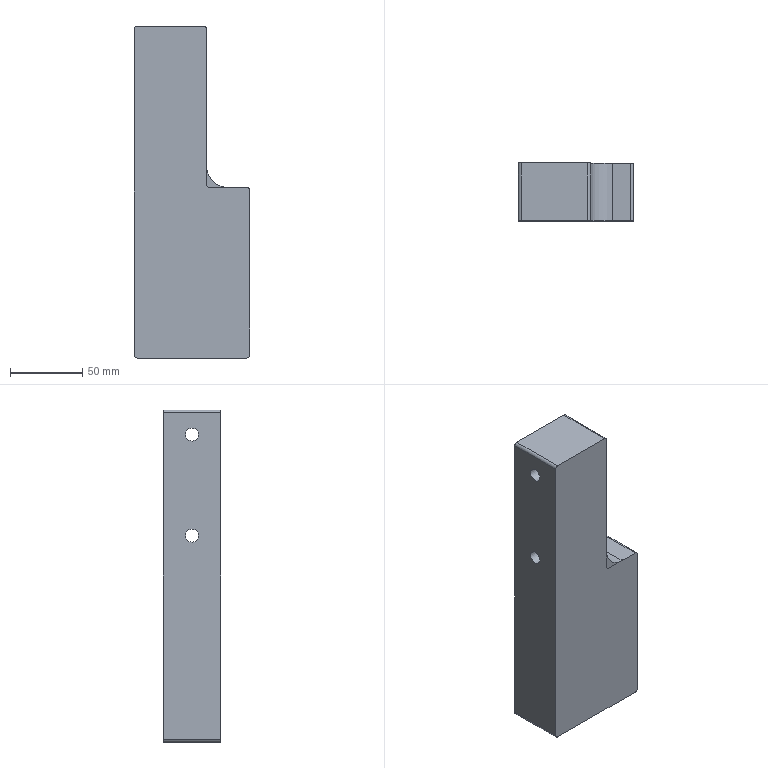NC program | NX | posted with a generic post | part box 80 x 40 x 230 mm
Whole program:
N10 G17 G21 G94 G90
(DRILLING_COPY , TOOL : D8点钻)
N12 T03 M6
N14 G53
N16 G17 G0 G90 X16. Y-10.9 B0. C0. S3500 M3
N18 G43 Z30. H3
N20 G94 G81 G98 Z-4.2 B-180. C-90. F300. R3.
N22 X106.
N24 X143. Y-20. Z-34.1 R-26.9
N26 X213.
N28 G80
N30 G0 X213. Y-20. Z30.
N32 M5
(PECK_DRILLING , TOOL : Z6.8)
N34 T10 M6
N36 G53
N38 G17 G0 G90 X16. Y-10.9 B0. C0. S1200 M3
N40 G43 Z50. H10
N42 G94 G83 G99 Z-33. B-180. C-90. F80. Q2. R3.
N44 X106.
N46 G80
N48 G0 X106. Y-10.9 Z50.
N50 M5
(PECK_DRILLING_COPY_1 , TOOL : Z9.)
N52 T24 M6
N54 G53
N56 G17 G0 G90 X143. Y-20. B0. C0. S1000 M3
N58 G43 Z50. H24
N60 G94 G83 G99 Z-85.9 B-180. C-90. F80. Q2. R-26.9
N62 X213.
N64 G80
N66 G0 X213. Y-20. Z50.
N68 M5
(HOLE_MILLING , TOOL : D6.)
N70 T05 M6
N72 G53
N74 G17 G0 G90 X143. Y-20. B0. C0. S2700 M3
N76 G43 Z50. H5
N78 Z-29.4 B-180. C-90.
N80 G94 G3 X140.765 Y-22.235 R2.235 F800.
N82 X143. Y-24.47 R2.235
N84 X143. Y-24.47 Z-29.65 I0. J4.47
N86 X143. Y-24.47 Z-29.9 I0. J4.47
N88 X143. Y-24.47 Z-30.15 I0. J4.47
N90 X143. Y-24.47 Z-30.4 I0. J4.47
N92 X143. Y-24.47 Z-30.65 I0. J4.47
N94 X143. Y-24.47 Z-30.9 I0. J4.47
N96 X143. Y-24.47 Z-31.15 I0. J4.47
N98 X143. Y-24.47 Z-31.4 I0. J4.47
N100 X143. Y-24.47 Z-31.65 I0. J4.47
N102 X143. Y-24.47 Z-31.9 I0. J4.47
N104 X143. Y-24.47 Z-32.15 I0. J4.47
N106 X143. Y-24.47 Z-32.4 I0. J4.47
N108 X143. Y-24.47 Z-32.65 I0. J4.47
N110 X143. Y-24.47 Z-32.9 I0. J4.47
N112 X143. Y-24.47 Z-33.15 I0. J4.47
N114 X143. Y-24.47 Z-33.4 I0. J4.47
N116 X143. Y-24.47 Z-33.65 I0. J4.47
N118 X143. Y-24.47 Z-33.9 I0. J4.47
N120 X143. Y-24.47 Z-34.15 I0. J4.47
N122 X143. Y-24.47 Z-34.4 I0. J4.47
N124 X143. Y-24.47 Z-34.65 I0. J4.47
N126 X143. Y-24.47 Z-34.9 I0. J4.47
N128 X143. Y-24.47 Z-35.15 I0. J4.47
N130 X143. Y-24.47 Z-35.4 I0. J4.47
N132 X143. Y-24.47 Z-35.65 I0. J4.47
N134 X143. Y-24.47 Z-35.9 I0. J4.47
N136 X143. Y-24.47 Z-36.15 I0. J4.47
N138 X143. Y-24.47 Z-36.4 I0. J4.47
N140 X143. Y-24.47 Z-36.65 I0. J4.47
N142 X143. Y-24.47 Z-36.9 I0. J4.47
N144 X143. Y-24.47 Z-37.15 I0. J4.47
N146 X143. Y-24.47 Z-37.4 I0. J4.47
N148 X143. Y-24.47 Z-37.65 I0. J4.47
N150 X143. Y-24.47 Z-37.9 I0. J4.47
N152 X143. Y-24.47 Z-38.15 I0. J4.47
N154 X143. Y-24.47 Z-38.4 I0. J4.47
N156 X143. Y-24.47 Z-38.65 I0. J4.47
N158 X143. Y-24.47 Z-38.9 I0. J4.47
N160 X143. Y-24.47 Z-39.15 I0. J4.47
N162 X143. Y-24.47 Z-39.4 I0. J4.47
N164 X143. Y-24.47 Z-39.65 I0. J4.47
N166 X143. Y-24.47 Z-39.9 I0. J4.47
N168 X143. Y-24.47 Z-40.15 I0. J4.47
N170 X143. Y-24.47 Z-40.4 I0. J4.47
N172 X143. Y-24.47 Z-40.65 I0. J4.47
N174 X143. Y-24.47 Z-40.9 I0. J4.47
N176 X143. Y-24.47 Z-41.15 I0. J4.47
N178 X143. Y-24.47 Z-41.4 I0. J4.47
N180 X143. Y-24.47 Z-41.65 I0. J4.47
N182 X143. Y-24.47 Z-41.9 I0. J4.47
N184 X143. Y-24.47 Z-42.15 I0. J4.47
N186 X143. Y-24.47 Z-42.4 I0. J4.47
N188 X143. Y-24.47 Z-42.65 I0. J4.47
N190 X143. Y-24.47 Z-42.9 I0. J4.47
N192 X143. Y-24.47 Z-43.15 I0. J4.47
N194 X143. Y-24.47 Z-43.4 I0. J4.47
N196 X143. Y-24.47 Z-43.65 I0. J4.47
N198 X143. Y-24.47 Z-43.9 I0. J4.47
N200 X143. Y-24.47 Z-44.15 I0. J4.47
N202 X143. Y-24.47 Z-44.4 I0. J4.47
N204 X143. Y-24.47 Z-44.65 I0. J4.47
N206 X143. Y-24.47 Z-44.9 I0. J4.47
N208 X147.251 Y-21.381 Z-44.95 R4.47
N210 X144.381 Y-15.749 R4.47
N212 X147.251 Y-21.381 R-4.47
N214 X145.816 Y-18.565 R2.235
N216 X143. Y-20. R2.235
N218 G0 Z50.
N220 X213.
N222 Z-29.4
N224 G3 X210.765 Y-22.235 R2.235
N226 X213. Y-24.47 R2.235
N228 X213. Y-24.47 Z-29.65 I0. J4.47
N230 X213. Y-24.47 Z-29.9 I0. J4.47
N232 X213. Y-24.47 Z-30.15 I0. J4.47
N234 X213. Y-24.47 Z-30.4 I0. J4.47
N236 X213. Y-24.47 Z-30.65 I0. J4.47
N238 X213. Y-24.47 Z-30.9 I0. J4.47
N240 X213. Y-24.47 Z-31.15 I0. J4.47
N242 X213. Y-24.47 Z-31.4 I0. J4.47
N244 X213. Y-24.47 Z-31.65 I0. J4.47
N246 X213. Y-24.47 Z-31.9 I0. J4.47
N248 X213. Y-24.47 Z-32.15 I0. J4.47
N250 X213. Y-24.47 Z-32.4 I0. J4.47
N252 X213. Y-24.47 Z-32.65 I0. J4.47
N254 X213. Y-24.47 Z-32.9 I0. J4.47
N256 X213. Y-24.47 Z-33.15 I0. J4.47
N258 X213. Y-24.47 Z-33.4 I0. J4.47
N260 X213. Y-24.47 Z-33.65 I0. J4.47
N262 X213. Y-24.47 Z-33.9 I0. J4.47
N264 X213. Y-24.47 Z-34.15 I0. J4.47
N266 X213. Y-24.47 Z-34.4 I0. J4.47
N268 X213. Y-24.47 Z-34.65 I0. J4.47
N270 X213. Y-24.47 Z-34.9 I0. J4.47
N272 X213. Y-24.47 Z-35.15 I0. J4.47
N274 X213. Y-24.47 Z-35.4 I0. J4.47
N276 X213. Y-24.47 Z-35.65 I0. J4.47
N278 X213. Y-24.47 Z-35.9 I0. J4.47
N280 X213. Y-24.47 Z-36.15 I0. J4.47
N282 X213. Y-24.47 Z-36.4 I0. J4.47
N284 X213. Y-24.47 Z-36.65 I0. J4.47
N286 X213. Y-24.47 Z-36.9 I0. J4.47
N288 X213. Y-24.47 Z-37.15 I0. J4.47
N290 X213. Y-24.47 Z-37.4 I0. J4.47
N292 X213. Y-24.47 Z-37.65 I0. J4.47
N294 X213. Y-24.47 Z-37.9 I0. J4.47
N296 X213. Y-24.47 Z-38.15 I0. J4.47
N298 X213. Y-24.47 Z-38.4 I0. J4.47
N300 X213. Y-24.47 Z-38.65 I0. J4.47
N302 X213. Y-24.47 Z-38.9 I0. J4.47
N304 X213. Y-24.47 Z-39.15 I0. J4.47
N306 X213. Y-24.47 Z-39.4 I0. J4.47
N308 X213. Y-24.47 Z-39.65 I0. J4.47
N310 X213. Y-24.47 Z-39.9 I0. J4.47
N312 X213. Y-24.47 Z-40.15 I0. J4.47
N314 X213. Y-24.47 Z-40.4 I0. J4.47
N316 X213. Y-24.47 Z-40.65 I0. J4.47
N318 X213. Y-24.47 Z-40.9 I0. J4.47
N320 X213. Y-24.47 Z-41.15 I0. J4.47
N322 X213. Y-24.47 Z-41.4 I0. J4.47
N324 X213. Y-24.47 Z-41.65 I0. J4.47
N326 X213. Y-24.47 Z-41.9 I0. J4.47
N328 X213. Y-24.47 Z-42.15 I0. J4.47
N330 X213. Y-24.47 Z-42.4 I0. J4.47
N332 X213. Y-24.47 Z-42.65 I0. J4.47
N334 X213. Y-24.47 Z-42.9 I0. J4.47
N336 X213. Y-24.47 Z-43.15 I0. J4.47
N338 X213. Y-24.47 Z-43.4 I0. J4.47
N340 X213. Y-24.47 Z-43.65 I0. J4.47
N342 X213. Y-24.47 Z-43.9 I0. J4.47
N344 X213. Y-24.47 Z-44.15 I0. J4.47
N346 X213. Y-24.47 Z-44.4 I0. J4.47
N348 X213. Y-24.47 Z-44.65 I0. J4.47
N350 X213. Y-24.47 Z-44.9 I0. J4.47
N352 X217.251 Y-21.381 Z-44.95 R4.47
N354 X214.381 Y-15.749 R4.47
N356 X217.251 Y-21.381 R-4.47
N358 X215.816 Y-18.565 R2.235
N360 X213. Y-20. R2.235
N362 G0 Z50.
(HOLE_MILLING_COPY , TOOL : D6.)
N364 X143. S3000
N366 Z-45.
N368 G3 X140.75 Y-22.25 R2.25 F60.
N370 X143. Y-24.5 R2.25
N372 X147.5 Y-20. R4.5
N374 X143. Y-24.5 R-4.5
N376 X145.25 Y-22.25 R2.25
N378 X143. Y-20. R2.25
N380 G0 Z50.
N382 X213.
N384 Z-45.
N386 G3 X210.75 Y-22.25 R2.25
N388 X213. Y-24.5 R2.25
N390 X217.5 Y-20. R4.5
N392 X213. Y-24.5 R-4.5
N394 X215.25 Y-22.25 R2.25
N396 X213. Y-20. R2.25
N398 G0 Z50.
N400 M5
(ZLEVEL_PROFILE_STEEP , TOOL : D16CU)
N402 T01 M6
N404 G53
N406 G17 G0 G90 X126.2 Y10.296 B0. C0. S2600 M3
N408 G43 Z50. H1
N410 Z-15.199 B-180. C-90.
N412 G94 G1 Y0. F2200.
N414 Y-40.
N416 Y-50.296
N418 G0 Z-15.397
N420 G1 Y-40.
N422 Y0.
N424 Y10.296
N426 G0 Z-15.596
N428 G1 Y0.
N430 Y-40.
N432 Y-50.296
N434 G0 Z-15.795
N436 G1 Y-40.
N438 Y0.
N440 Y10.296
N442 G0 Z-15.993
N444 G1 Y0.
N446 Y-40.
N448 Y-50.296
N450 G0 Z-16.192
N452 G1 Y-40.
N454 Y0.
N456 Y10.296
N458 G0 Z-16.391
N460 G1 Y0.
N462 Y-40.
N464 Y-50.296
N466 G0 Z-16.589
N468 G1 Y-40.
N470 Y0.
N472 Y10.296
N474 G0 Z-16.788
N476 G1 Y0.
N478 Y-40.
N480 Y-50.296
N482 G0 Z-16.987
N484 G1 Y-40.
N486 Y0.
N488 Y10.296
N490 G0 Z-17.185
N492 G1 Y0.
N494 Y-40.
N496 Y-50.296
N498 G0 Z-17.384
N500 G1 Y-40.
N502 Y0.
N504 Y10.296
N506 G0 Z-17.583
N508 G1 Y0.
N510 Y-40.
N512 Y-50.296
N514 G0 Z-17.781
N516 G1 Y-40.
N518 Y0.
N520 Y10.296
N522 G0 Z-17.98
N524 G1 Y0.
N526 Y-40.
N528 Y-50.296
N530 G0 Z-18.179
N532 G1 Y-40.
N534 Y0.
N536 Y10.296
N538 G0 Z-18.377
N540 G1 Y0.
N542 Y-40.
N544 Y-50.296
N546 G0 Z-18.576
N548 G1 Y-40.
N550 Y0.
N552 Y10.296
N554 G0 Z-18.775
N556 G1 Y0.
N558 Y-40.
N560 Y-50.296
N562 G0 Z-18.973
N564 G1 Y-40.
N566 Y0.
N568 Y10.296
N570 G0 Z-19.172
N572 G1 Y0.
N574 Y-40.
N576 Y-50.296
N578 G0 Z-19.371
N580 G1 Y-40.
N582 Y0.
N584 Y10.296
N586 G0 Z-19.569
N588 G1 Y0.
N590 Y-40.
N592 Y-50.296
N594 G0 Z-19.768
N596 G1 Y-40.
N598 Y0.
N600 Y10.296
N602 G0 Z-19.967
N604 G1 Y0.
N606 Y-40.
N608 Y-50.296
N610 G0 Z-20.165
N612 G1 Y-40.
N614 Y0.
N616 Y10.296
N618 G0 Z-20.364
N620 G1 Y0.
N622 Y-40.
N624 Y-50.296
N626 G0 Z-20.563
N628 G1 Y-40.
N630 Y0.
N632 Y10.296
N634 G0 Z-20.761
N636 G1 Y0.
N638 Y-40.
N640 Y-50.296
N642 G0 Z-20.96
N644 G1 Y-40.
N646 Y0.
N648 Y10.296
N650 G0 Z-21.159
N652 G1 Y0.
N654 Y-40.
N656 Y-50.296
N658 G0 Z-21.357
N660 G1 Y-40.
N662 Y0.
N664 Y10.296
N666 G0 Z-21.556
N668 G1 Y0.
N670 Y-40.
N672 Y-50.296
N674 G0 Z-21.755
N676 G1 Y-40.
N678 Y0.
N680 Y10.296
N682 G0 Z-21.953
N684 G1 Y0.
N686 Y-40.
N688 Y-50.296
N690 G0 Z-22.152
N692 G1 Y-40.
N694 Y0.
N696 Y10.296
N698 G0 Z-22.351
N700 G1 Y0.
N702 Y-40.
N704 Y-50.296
N706 G0 Z-22.549
N708 G1 Y-40.
N710 Y0.
N712 Y10.296
N714 G0 Z-22.748
N716 G1 Y0.
N718 Y-40.
N720 Y-50.296
N722 G0 Z-22.947
N724 G1 Y-40.
N726 Y0.
N728 Y10.296
N730 G0 Z-23.145
N732 G1 Y0.
N734 Y-40.
N736 Y-50.296
N738 G0 Z-23.344
N740 G1 Y-40.
N742 Y0.
N744 Y10.296
N746 G0 Z-23.543
N748 G1 Y0.
N750 Y-40.
N752 Y-50.296
N754 G0 Z-23.741
N756 G1 Y-40.
N758 Y0.
N760 Y10.296
N762 G0 Z-23.94
N764 G1 Y0.
N766 Y-40.
N768 Y-50.296
N770 G0 Z-24.139
N772 G1 Y-40.
N774 Y0.
N776 Y10.296
N778 G0 Z-24.337
N780 G1 Y0.
N782 Y-40.
N784 Y-50.296
N786 G0 Z-24.536
N788 G1 Y-40.
N790 Y0.
N792 Y10.296
N794 G0 Z-24.735
N796 G1 Y0.
N798 Y-40.
N800 Y-50.296
N802 G0 Z-24.933
N804 G1 Y-40.
N806 Y0.
N808 Y10.296
N810 G0 Z-25.132
N812 G1 Y0.
N814 Y-40.
N816 Y-50.296
N818 G0 Z-25.331
N820 G1 Y-40.
N822 Y0.
N824 Y10.296
N826 G0 Z-25.529
N828 G1 Y0.
N830 Y-40.
N832 Y-50.296
N834 G0 Z-25.728
N836 G1 Y-40.
N838 Y0.
N840 Y10.296
N842 G0 Z-25.927
N844 G1 Y0.
N846 Y-40.
N848 Y-50.296
N850 G0 Z-26.125
N852 G1 Y-40.
N854 Y0.
N856 Y10.296
N858 G0 Z-26.324
N860 G1 Y0.
N862 Y-40.
N864 Y-50.296
N866 G0 Z-26.523
N868 G1 Y-40.
N870 Y0.
N872 Y10.296
N874 G0 Z-26.721
N876 G1 Y0.
N878 Y-40.
N880 Y-50.296
N882 G0 Z-26.92
N884 G1 Y-40.
N886 Y0.
N888 Y10.296
N890 G0 Z-27.119
N892 G1 Y0.
N894 Y-40.
N896 Y-50.296
N898 G0 Z-27.317
N900 G1 Y-40.
N902 Y0.
N904 Y10.296
N906 G0 Z-27.516
N908 G1 Y0.
N910 Y-40.
N912 Y-50.296
N914 G0 Z-27.715
N916 G1 Y-40.
N918 Y0.
N920 Y10.296
N922 G0 Y10.297 Z-27.913
N924 G1 Y-0.069
N926 Y-39.925
N928 Y-50.297
N930 G0 X126.218 Y-50.306 Z-28.112
N932 G1 Y-39.981
N934 X126.212 Y-39.963
N936 Y-0.011
N938 Y10.315
N940 G0 X126.245 Y10.317 Z-28.311
N942 G1 Y0.
N944 Y-40.
N946 Y-50.314
N948 G0 X126.3 Y-50.306 Z-28.509
N950 G1 Y-40.
N952 Y0.
N954 Y10.301
N956 G0 X126.38 Y10.331 Z-28.708
N958 G1 Y-0.072
N960 Y-39.922
N962 Y-50.33
N964 G0 X126.489 Y-50.311 Z-28.907
N966 G1 Y-40.
N968 Y0.002
N970 Y10.326
N972 G0 X126.631 Y10.321 Z-29.105
N974 G1 Y0.
N976 Y-40.
N978 Y-50.316
N980 G0 X126.82 Y-50.322 Z-29.304
N982 G1 Y-40.
N984 Y0.
N986 Y10.319
N988 G0 X127.079 Y10.315 Z-29.503
N990 G1 Y0.
N992 Y-40.
N994 Y-50.319
N996 G0 X127.496 Y-50.32 Z-29.701
N998 G1 Y-40.
N1000 Y0.
N1002 Y10.309
N1004 G0 Z50.
N1006 M5
(PLANAR_MILL , TOOL : D10R2.)
N1008 T23 M6
N1010 G53
N1012 G17 G0 G90 X123.12 Y10. B0. C0. S2400 M3
N1014 G43 Z50. H23
N1016 Z-11.9 B-180. C-90.
N1018 G94 G1 Z-14.9 F400.
N1020 Y0.
N1022 Y-40.
N1024 Y-50.
N1026 Z-11.9
N1028 G0 Z50.
N1030 X123.1 Y10.
N1032 Z-11.9
N1034 G1 Z-14.9
N1036 Y0.
N1038 Y-40.
N1040 Y-50.
N1042 Z-11.9
N1044 G0 Z50.
(PLANAR_MILL_COPY_2 , TOOL : D10R2.)
N1046 X123.125 Y10.
N1048 Z-26.9
N1050 G1 Z-29.9
N1052 Y0.
N1054 Y-40.
N1056 Y-50.
N1058 Z-26.9
N1060 G0 Z50.
N1062 X123.105 Y10.
N1064 Z-26.9
N1066 G1 Z-29.9
N1068 Y0.
N1070 Y-40.
N1072 Y-50.
N1074 Z-26.9
N1076 G0 Z50.
(PLANAR_MILL_COPY_1 , TOOL : D10R2.)
N1078 X228.105 Y8.
N1080 Z-29.7
N1082 G1 Z-29.9
N1084 Y0.
N1086 Y-40.
N1088 Y-48.
N1090 Z-29.7
N1092 G0 X223.105 Y8.
N1094 G1 Z-29.9
N1096 Y0.
N1098 Y-40.
N1100 Y-48.
N1102 Z-29.7
N1104 G0 X218.105 Y8.
N1106 G1 Z-29.9
N1108 Y0.
N1110 Y-40.
N1112 Y-48.
N1114 Z-29.7
N1116 G0 X213.105 Y8.
N1118 G1 Z-29.9
N1120 Y0.
N1122 Y-40.
N1124 Y-48.
N1126 Z-29.7
N1128 G0 X208.105 Y8.
N1130 G1 Z-29.9
N1132 Y0.
N1134 Y-40.
N1136 Y-48.
N1138 Z-29.7
N1140 G0 X203.105 Y8.
N1142 G1 Z-29.9
N1144 Y0.
N1146 Y-40.
N1148 Y-48.
N1150 Z-29.7
N1152 G0 X198.105 Y8.
N1154 G1 Z-29.9
N1156 Y0.
N1158 Y-40.
N1160 Y-48.
N1162 Z-29.7
N1164 G0 X193.105 Y8.
N1166 G1 Z-29.9
N1168 Y0.
N1170 Y-40.
N1172 Y-48.
N1174 Z-29.7
N1176 G0 X188.105 Y8.
N1178 G1 Z-29.9
N1180 Y0.
N1182 Y-40.
N1184 Y-48.
N1186 Z-29.7
N1188 G0 X183.105 Y8.
N1190 G1 Z-29.9
N1192 Y0.
N1194 Y-40.
N1196 Y-48.
N1198 Z-29.7
N1200 G0 X178.105 Y8.
N1202 G1 Z-29.9
N1204 Y0.
N1206 Y-40.
N1208 Y-48.
N1210 Z-29.7
N1212 G0 X173.105 Y8.
N1214 G1 Z-29.9
N1216 Y0.
N1218 Y-40.
N1220 Y-48.
N1222 Z-29.7
N1224 G0 X168.105 Y8.
N1226 G1 Z-29.9
N1228 Y0.
N1230 Y-40.
N1232 Y-48.
N1234 Z-29.7
N1236 G0 X163.105 Y8.
N1238 G1 Z-29.9
N1240 Y0.
N1242 Y-40.
N1244 Y-48.
N1246 Z-29.7
N1248 G0 X158.105 Y8.
N1250 G1 Z-29.9
N1252 Y0.
N1254 Y-40.
N1256 Y-48.
N1258 Z-29.7
N1260 G0 X153.105 Y8.
N1262 G1 Z-29.9
N1264 Y0.
N1266 Y-40.
N1268 Y-48.
N1270 Z-29.7
N1272 G0 X148.105 Y8.
N1274 G1 Z-29.9
N1276 Y0.
N1278 Y-40.
N1280 Y-48.
N1282 Z-29.7
N1284 G0 X143.105 Y8.
N1286 G1 Z-29.9
N1288 Y0.
N1290 Y-40.
N1292 Y-48.
N1294 Z-29.7
N1296 G0 X138.105 Y8.
N1298 G1 Z-29.9
N1300 Y0.
N1302 Y-40.
N1304 Y-48.
N1306 Z-29.7
N1308 G0 X133.105 Y8.
N1310 G1 Z-29.9
N1312 Y0.
N1314 Y-40.
N1316 Y-48.
N1318 Z-29.7
N1320 G0 X128.105 Y8.
N1322 G1 Z-29.9
N1324 Y0.
N1326 Y-40.
N1328 Y-48.
N1330 Z-29.7
N1332 G0 X123.105 Y8.
N1334 G1 Z-29.9
N1336 Y0.
N1338 Y-40.
N1340 Y-48.
N1342 Z-29.7
N1344 G0 Z50.
N1346 M5
N1348 M2